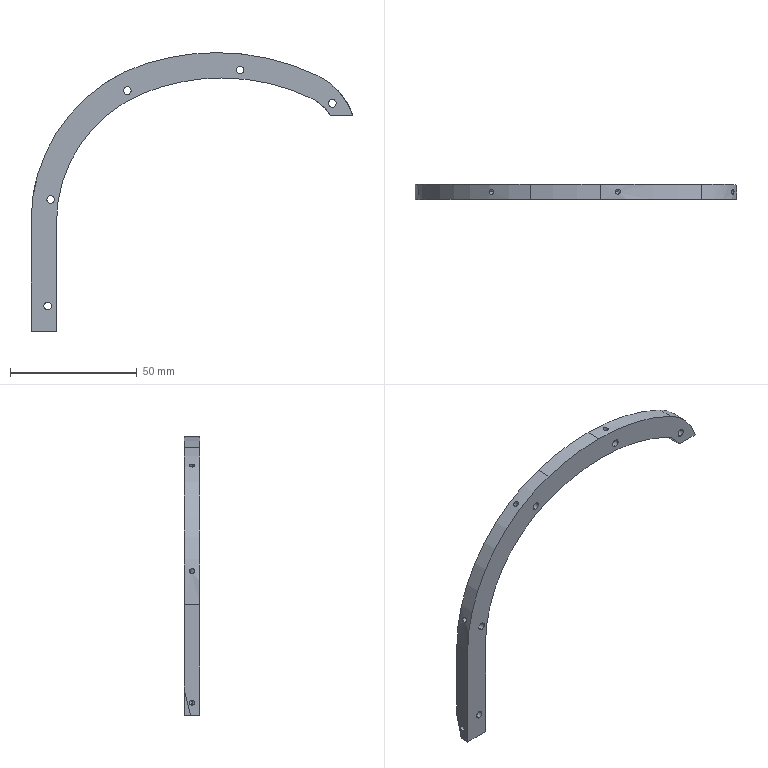Part | SolidWorks | features ICE 3, Cut 2, 3DProfileFeature 1, Chamfer 1, CurvePattern 1, Extrusion 1, HoleWzd 1 | 1 solid | 47 faces | box 126.964 x 6 x 110 mm | volume 11727 mm3 | cylinder 28 | cone 10 | plane 9 | commonest cylinder face diameters 2.05 x10 3 x10 164.469 x2 184.469 x2 33 x1 53 x1